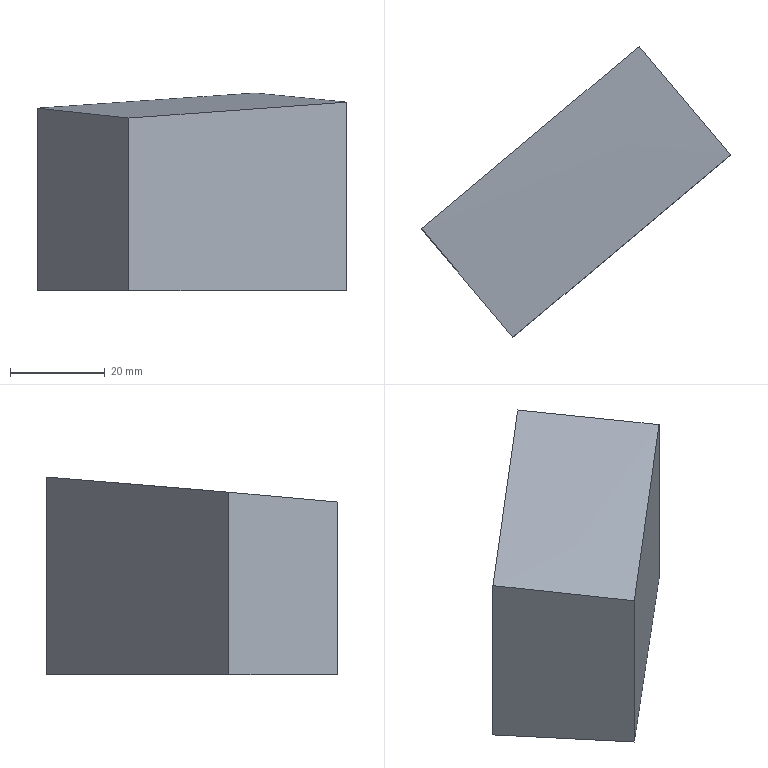Part | NX | features solid 2 | 1 solid | 6 faces | box 65.246 x 61.549 x 41.855 mm | volume 70698 mm3 | plane 5 | spline 1
STEP:
#1=CARTESIAN_POINT('',(-307.06,-342.827,15.));
#2=VERTEX_POINT('',#1);
#3=CARTESIAN_POINT('',(-261.097,-304.259,15.));
#4=VERTEX_POINT('',#3);
#5=CARTESIAN_POINT('',(-299.399,-336.399,15.));
#6=DIRECTION('',(-0.766,-0.6428,0.));
#7=VECTOR('',#6,1000.);
#8=LINE('',#5,#7);
#9=EDGE_CURVE('',#2,#4,#8,.F.);
#10=ORIENTED_EDGE('',*,*,#9,.T.);
#11=CARTESIAN_POINT('',(-241.813,-327.241,15.));
#12=VERTEX_POINT('',#11);
#13=CARTESIAN_POINT('',(-261.097,-304.259,15.));
#14=DIRECTION('',(-0.6428,0.766,0.));
#15=VECTOR('',#14,1000.);
#16=LINE('',#13,#15);
#17=EDGE_CURVE('',#4,#12,#16,.F.);
#18=ORIENTED_EDGE('',*,*,#17,.T.);
#19=CARTESIAN_POINT('',(-287.776,-365.808,15.));
#20=VERTEX_POINT('',#19);
#21=CARTESIAN_POINT('',(-280.115,-359.38,15.));
#22=DIRECTION('',(0.766,0.6428,0.));
#23=VECTOR('',#22,1000.);
#24=LINE('',#21,#23);
#25=EDGE_CURVE('',#20,#12,#24,.T.);
#26=ORIENTED_EDGE('',*,*,#25,.F.);
#27=CARTESIAN_POINT('',(-307.06,-342.827,15.));
#28=DIRECTION('',(-0.6428,0.766,0.));
#29=VECTOR('',#28,1000.);
#30=LINE('',#27,#29);
#31=EDGE_CURVE('',#2,#20,#30,.F.);
#32=ORIENTED_EDGE('',*,*,#31,.F.);
#33=EDGE_LOOP('',(#10,#18,#26,#32));
#34=FACE_BOUND('',#33,.T.);
#35=CARTESIAN_POINT('',(-299.399,-336.399,15.));
#36=DIRECTION('',(0.,0.,-1.));
#37=DIRECTION('',(0.6428,-0.766,0.));
#38=AXIS2_PLACEMENT_3D('',#35,#36,#37);
#39=PLANE('',#38);
#40=ADVANCED_FACE('',(#34),#39,.T.);
#41=CARTESIAN_POINT('',(-241.813,-327.241,54.917));
#42=VERTEX_POINT('',#41);
#43=CARTESIAN_POINT('',(-241.813,-327.241,-50.));
#44=DIRECTION('',(0.,0.,-1.));
#45=VECTOR('',#44,1000.);
#46=LINE('',#43,#45);
#47=EDGE_CURVE('',#12,#42,#46,.F.);
#48=ORIENTED_EDGE('',*,*,#47,.T.);
#49=CARTESIAN_POINT('',(-287.776,-365.808,51.56));
#50=VERTEX_POINT('',#49);
#51=CARTESIAN_POINT('',(-241.813,-327.241,54.917));
#52=CARTESIAN_POINT('',(-257.136,-340.098,53.844));
#53=CARTESIAN_POINT('',(-272.457,-352.954,52.726));
#54=CARTESIAN_POINT('',(-287.776,-365.808,51.56));
#55=B_SPLINE_CURVE_WITH_KNOTS('',3,(#51,#52,#53,#54),.UNSPECIFIED.,.F.,.F.,(4,4),(0.3354,0.3955),.UNSPECIFIED.);
#56=EDGE_CURVE('',#42,#50,#55,.T.);
#57=ORIENTED_EDGE('',*,*,#56,.T.);
#58=CARTESIAN_POINT('',(-287.776,-365.808,-50.));
#59=DIRECTION('',(0.,0.,-1.));
#60=VECTOR('',#59,1000.);
#61=LINE('',#58,#60);
#62=EDGE_CURVE('',#20,#50,#61,.F.);
#63=ORIENTED_EDGE('',*,*,#62,.F.);
#64=ORIENTED_EDGE('',*,*,#25,.T.);
#65=EDGE_LOOP('',(#48,#57,#63,#64));
#66=FACE_BOUND('',#65,.T.);
#67=CARTESIAN_POINT('',(-280.115,-359.38,-50.));
#68=DIRECTION('',(0.6428,-0.766,0.));
#69=DIRECTION('',(0.,0.,1.));
#70=AXIS2_PLACEMENT_3D('',#67,#68,#69);
#71=PLANE('',#70);
#72=ADVANCED_FACE('',(#66),#71,.T.);
#73=CARTESIAN_POINT('',(-307.06,-342.827,53.649));
#74=VERTEX_POINT('',#73);
#75=CARTESIAN_POINT('',(-307.06,-342.827,-50.));
#76=DIRECTION('',(0.,0.,1.));
#77=VECTOR('',#76,1000.);
#78=LINE('',#75,#77);
#79=EDGE_CURVE('',#2,#74,#78,.T.);
#80=ORIENTED_EDGE('',*,*,#79,.T.);
#81=CARTESIAN_POINT('',(-261.097,-304.259,56.855));
#82=VERTEX_POINT('',#81);
#83=CARTESIAN_POINT('',(-307.06,-342.827,53.649));
#84=CARTESIAN_POINT('',(-291.741,-329.972,54.763));
#85=CARTESIAN_POINT('',(-276.42,-317.117,55.831));
#86=CARTESIAN_POINT('',(-261.097,-304.259,56.855));
#87=B_SPLINE_CURVE_WITH_KNOTS('',3,(#83,#84,#85,#86),.UNSPECIFIED.,.F.,.F.,(4,4),(0.09163,0.1517),.UNSPECIFIED.);
#88=EDGE_CURVE('',#74,#82,#87,.T.);
#89=ORIENTED_EDGE('',*,*,#88,.T.);
#90=CARTESIAN_POINT('',(-261.097,-304.259,-50.));
#91=DIRECTION('',(0.,0.,1.));
#92=VECTOR('',#91,1000.);
#93=LINE('',#90,#92);
#94=EDGE_CURVE('',#4,#82,#93,.T.);
#95=ORIENTED_EDGE('',*,*,#94,.F.);
#96=ORIENTED_EDGE('',*,*,#9,.F.);
#97=EDGE_LOOP('',(#80,#89,#95,#96));
#98=FACE_BOUND('',#97,.T.);
#99=CARTESIAN_POINT('',(-299.399,-336.399,-50.));
#100=DIRECTION('',(0.6428,-0.766,0.));
#101=DIRECTION('',(0.,0.,1.));
#102=AXIS2_PLACEMENT_3D('',#99,#100,#101);
#103=PLANE('',#102);
#104=ADVANCED_FACE('',(#98),#103,.F.);
#105=ORIENTED_EDGE('',*,*,#94,.T.);
#106=CARTESIAN_POINT('',(-261.097,-304.259,56.855));
#107=CARTESIAN_POINT('',(-254.668,-311.921,56.226));
#108=CARTESIAN_POINT('',(-248.24,-319.581,55.58));
#109=CARTESIAN_POINT('',(-241.813,-327.241,54.917));
#110=B_SPLINE_CURVE_WITH_KNOTS('',3,(#106,#107,#108,#109),.UNSPECIFIED.,.F.,.F.,(4,4),(0.1719,0.202),.UNSPECIFIED.);
#111=EDGE_CURVE('',#82,#42,#110,.T.);
#112=ORIENTED_EDGE('',*,*,#111,.T.);
#113=ORIENTED_EDGE('',*,*,#47,.F.);
#114=ORIENTED_EDGE('',*,*,#17,.F.);
#115=EDGE_LOOP('',(#105,#112,#113,#114));
#116=FACE_BOUND('',#115,.T.);
#117=CARTESIAN_POINT('',(-261.097,-304.259,-50.));
#118=DIRECTION('',(-0.766,-0.6428,0.));
#119=DIRECTION('',(0.6428,-0.766,0.));
#120=AXIS2_PLACEMENT_3D('',#117,#118,#119);
#121=PLANE('',#120);
#122=ADVANCED_FACE('',(#116),#121,.F.);
#123=CARTESIAN_POINT('',(-307.06,-342.827,53.649));
#124=CARTESIAN_POINT('',(-300.631,-350.488,52.97));
#125=CARTESIAN_POINT('',(-294.203,-358.148,52.274));
#126=CARTESIAN_POINT('',(-287.776,-365.808,51.56));
#127=B_SPLINE_CURVE_WITH_KNOTS('',3,(#123,#124,#125,#126),.UNSPECIFIED.,.F.,.F.,(4,4),(0.,0.03007),.UNSPECIFIED.);
#128=EDGE_CURVE('',#74,#50,#127,.T.);
#129=ORIENTED_EDGE('',*,*,#128,.F.);
#130=ORIENTED_EDGE('',*,*,#79,.F.);
#131=ORIENTED_EDGE('',*,*,#31,.T.);
#132=ORIENTED_EDGE('',*,*,#62,.T.);
#133=EDGE_LOOP('',(#129,#130,#131,#132));
#134=FACE_BOUND('',#133,.T.);
#135=CARTESIAN_POINT('',(-307.06,-342.827,-50.));
#136=DIRECTION('',(-0.766,-0.6428,0.));
#137=DIRECTION('',(0.6428,-0.766,0.));
#138=AXIS2_PLACEMENT_3D('',#135,#136,#137);
#139=PLANE('',#138);
#140=ADVANCED_FACE('',(#134),#139,.T.);
#141=ORIENTED_EDGE('',*,*,#88,.F.);
#142=ORIENTED_EDGE('',*,*,#128,.T.);
#143=ORIENTED_EDGE('',*,*,#56,.F.);
#144=ORIENTED_EDGE('',*,*,#111,.F.);
#145=EDGE_LOOP('',(#141,#142,#143,#144));
#146=FACE_BOUND('',#145,.T.);
#147=CARTESIAN_POINT('',(-241.403,-304.5,56.81));
#148=CARTESIAN_POINT('',(-263.409,-303.814,56.896));
#149=CARTESIAN_POINT('',(-285.419,-303.126,56.976));
#150=CARTESIAN_POINT('',(-307.432,-302.437,57.049));
#151=CARTESIAN_POINT('',(-241.421,-325.488,55.105));
#152=CARTESIAN_POINT('',(-263.424,-324.826,55.195));
#153=CARTESIAN_POINT('',(-285.431,-324.161,55.278));
#154=CARTESIAN_POINT('',(-307.442,-323.496,55.354));
#155=CARTESIAN_POINT('',(-241.437,-346.481,53.282));
#156=CARTESIAN_POINT('',(-263.438,-345.842,53.374));
#157=CARTESIAN_POINT('',(-285.443,-345.202,53.459));
#158=CARTESIAN_POINT('',(-307.452,-344.561,53.537));
#159=CARTESIAN_POINT('',(-241.452,-367.478,51.339));
#160=CARTESIAN_POINT('',(-263.451,-366.863,51.433));
#161=CARTESIAN_POINT('',(-285.454,-366.248,51.519));
#162=CARTESIAN_POINT('',(-307.461,-365.631,51.598));
#163=B_SPLINE_SURFACE_WITH_KNOTS('',3,3,((#147,#148,#149,#150),(#151,#152,#153,#154),(#155,#156,#157,#158),(#159,#160,#161,#162)),.UNSPECIFIED.,.F.,.F.,.F.,(4,4),(4,4),(0.2148,0.3049),(0.8002,0.8556),.UNSPECIFIED.);
#164=ADVANCED_FACE('',(#146),#163,.F.);
#165=CLOSED_SHELL('',(#40,#72,#104,#122,#140,#164));
#166=MANIFOLD_SOLID_BREP('',#165);
#167=(LENGTH_UNIT()NAMED_UNIT(*)SI_UNIT(.MILLI.,.METRE.));
#168=UNCERTAINTY_MEASURE_WITH_UNIT(LENGTH_MEASURE(0.0508),#167,'','');
#169=(NAMED_UNIT(*)PLANE_ANGLE_UNIT()SI_UNIT($,.RADIAN.));
#170=(NAMED_UNIT(*)SI_UNIT($,.STERADIAN.)SOLID_ANGLE_UNIT());
#171=(GEOMETRIC_REPRESENTATION_CONTEXT(3)GLOBAL_UNCERTAINTY_ASSIGNED_CONTEXT((#168))GLOBAL_UNIT_ASSIGNED_CONTEXT((#167,#169,#170))REPRESENTATION_CONTEXT('',''));
#172=ADVANCED_BREP_SHAPE_REPRESENTATION('',(#166),#171);